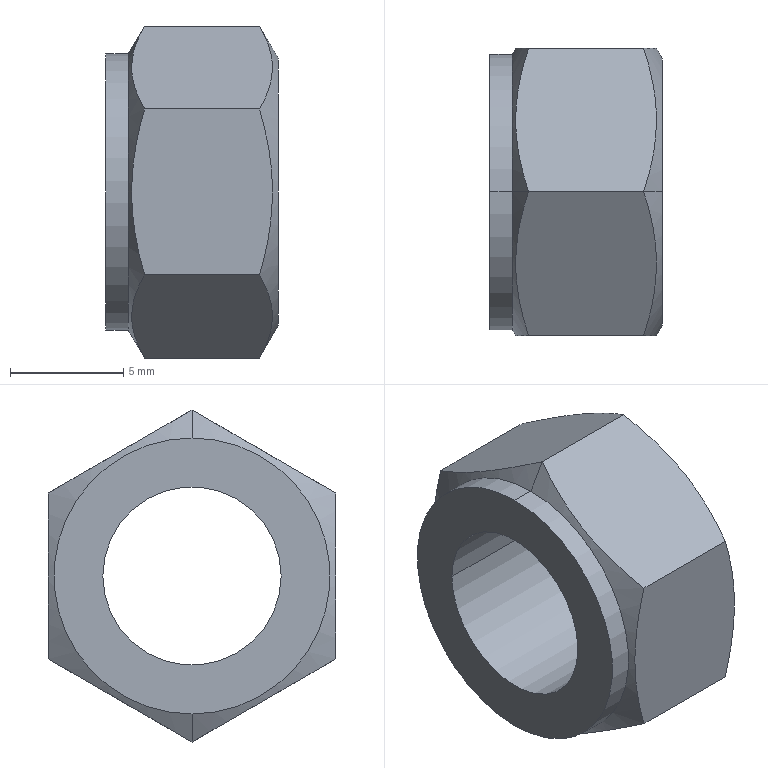Part | NX | features BREP 1 | 1 solid | 16 faces | box 7.62 x 12.7 x 14.665 mm | volume 657.652 mm3 | plane 8 | cylinder 4 | cone 4 | commonest cylinder face diameters 7.874 x2 12.192 x2
STEP:
#1=CARTESIAN_POINT('',(6.731,0.,5.903));
#2=VERTEX_POINT('',#1);
#3=CARTESIAN_POINT('',(6.731,0.,-5.903));
#4=VERTEX_POINT('',#3);
#5=CARTESIAN_POINT('',(6.731,0.,0.));
#6=DIRECTION('',(-1.,0.,0.));
#7=DIRECTION('',(0.,0.,1.));
#8=AXIS2_PLACEMENT_3D('',#5,#6,#7);
#9=CIRCLE('',#8,5.903);
#10=EDGE_CURVE('',#2,#4,#9,.T.);
#11=ORIENTED_EDGE('',*,*,#10,.F.);
#12=CARTESIAN_POINT('',(6.731,0.,0.));
#13=DIRECTION('',(-1.,0.,0.));
#14=DIRECTION('',(0.,0.,-1.));
#15=AXIS2_PLACEMENT_3D('',#12,#13,#14);
#16=CIRCLE('',#15,5.903);
#17=EDGE_CURVE('',#4,#2,#16,.T.);
#18=ORIENTED_EDGE('',*,*,#17,.F.);
#19=EDGE_LOOP('',(#11,#18));
#20=FACE_BOUND('',#19,.T.);
#21=CARTESIAN_POINT('',(6.731,-3.937,0.));
#22=VERTEX_POINT('',#21);
#23=CARTESIAN_POINT('',(6.731,3.937,0.));
#24=VERTEX_POINT('',#23);
#25=CARTESIAN_POINT('',(6.731,0.,0.));
#26=DIRECTION('',(1.,0.,0.));
#27=DIRECTION('',(0.,-1.,0.));
#28=AXIS2_PLACEMENT_3D('',#25,#26,#27);
#29=CIRCLE('',#28,3.937);
#30=EDGE_CURVE('',#22,#24,#29,.T.);
#31=ORIENTED_EDGE('',*,*,#30,.F.);
#32=CARTESIAN_POINT('',(6.731,0.,0.));
#33=DIRECTION('',(1.,0.,0.));
#34=DIRECTION('',(0.,1.,0.));
#35=AXIS2_PLACEMENT_3D('',#32,#33,#34);
#36=CIRCLE('',#35,3.937);
#37=EDGE_CURVE('',#24,#22,#36,.T.);
#38=ORIENTED_EDGE('',*,*,#37,.F.);
#39=EDGE_LOOP('',(#31,#38));
#40=FACE_BOUND('',#39,.T.);
#41=CARTESIAN_POINT('',(6.731,0.,0.));
#42=DIRECTION('',(1.,0.,0.));
#43=DIRECTION('',(0.,1.,0.));
#44=AXIS2_PLACEMENT_3D('',#41,#42,#43);
#45=PLANE('',#44);
#46=ADVANCED_FACE('',(#20,#40),#45,.T.);
#47=ORIENTED_EDGE('',*,*,#37,.T.);
#48=CARTESIAN_POINT('',(-0.889,-3.937,0.));
#49=VERTEX_POINT('',#48);
#50=CARTESIAN_POINT('',(-0.889,-3.937,0.));
#51=DIRECTION('',(1.,0.,0.));
#52=VECTOR('',#51,1000.);
#53=LINE('',#50,#52);
#54=EDGE_CURVE('',#22,#49,#53,.F.);
#55=ORIENTED_EDGE('',*,*,#54,.T.);
#56=CARTESIAN_POINT('',(-0.889,3.937,0.));
#57=VERTEX_POINT('',#56);
#58=CARTESIAN_POINT('',(-0.889,0.,0.));
#59=DIRECTION('',(1.,0.,0.));
#60=DIRECTION('',(0.,1.,0.));
#61=AXIS2_PLACEMENT_3D('',#58,#59,#60);
#62=CIRCLE('',#61,3.937);
#63=EDGE_CURVE('',#57,#49,#62,.T.);
#64=ORIENTED_EDGE('',*,*,#63,.F.);
#65=CARTESIAN_POINT('',(-0.889,3.937,0.));
#66=DIRECTION('',(1.,0.,0.));
#67=VECTOR('',#66,1000.);
#68=LINE('',#65,#67);
#69=EDGE_CURVE('',#24,#57,#68,.F.);
#70=ORIENTED_EDGE('',*,*,#69,.F.);
#71=EDGE_LOOP('',(#47,#55,#64,#70));
#72=FACE_BOUND('',#71,.T.);
#73=CARTESIAN_POINT('',(-1.651,0.,0.));
#74=DIRECTION('',(1.,0.,0.));
#75=DIRECTION('',(0.,1.,0.));
#76=AXIS2_PLACEMENT_3D('',#73,#74,#75);
#77=CYLINDRICAL_SURFACE('',#76,3.937);
#78=ADVANCED_FACE('',(#72),#77,.F.);
#79=CARTESIAN_POINT('',(-0.889,0.,0.));
#80=DIRECTION('',(1.,0.,0.));
#81=DIRECTION('',(0.,-1.,0.));
#82=AXIS2_PLACEMENT_3D('',#79,#80,#81);
#83=CIRCLE('',#82,3.937);
#84=EDGE_CURVE('',#49,#57,#83,.T.);
#85=ORIENTED_EDGE('',*,*,#84,.F.);
#86=ORIENTED_EDGE('',*,*,#54,.F.);
#87=ORIENTED_EDGE('',*,*,#30,.T.);
#88=ORIENTED_EDGE('',*,*,#69,.T.);
#89=EDGE_LOOP('',(#85,#86,#87,#88));
#90=FACE_BOUND('',#89,.T.);
#91=CARTESIAN_POINT('',(-1.651,0.,0.));
#92=DIRECTION('',(1.,0.,0.));
#93=DIRECTION('',(0.,1.,0.));
#94=AXIS2_PLACEMENT_3D('',#91,#92,#93);
#95=CYLINDRICAL_SURFACE('',#94,3.937);
#96=ADVANCED_FACE('',(#90),#95,.F.);
#97=CARTESIAN_POINT('',(-0.889,0.,6.096));
#98=VERTEX_POINT('',#97);
#99=CARTESIAN_POINT('',(-0.889,0.,-6.096));
#100=VERTEX_POINT('',#99);
#101=CARTESIAN_POINT('',(-0.889,0.,0.));
#102=DIRECTION('',(-1.,0.,0.));
#103=DIRECTION('',(0.,0.,1.));
#104=AXIS2_PLACEMENT_3D('',#101,#102,#103);
#105=CIRCLE('',#104,6.096);
#106=EDGE_CURVE('',#98,#100,#105,.T.);
#107=ORIENTED_EDGE('',*,*,#106,.T.);
#108=CARTESIAN_POINT('',(-0.889,0.,0.));
#109=DIRECTION('',(-1.,0.,0.));
#110=DIRECTION('',(0.,0.,-1.));
#111=AXIS2_PLACEMENT_3D('',#108,#109,#110);
#112=CIRCLE('',#111,6.096);
#113=EDGE_CURVE('',#100,#98,#112,.T.);
#114=ORIENTED_EDGE('',*,*,#113,.T.);
#115=EDGE_LOOP('',(#107,#114));
#116=FACE_BOUND('',#115,.T.);
#117=ORIENTED_EDGE('',*,*,#84,.T.);
#118=ORIENTED_EDGE('',*,*,#63,.T.);
#119=EDGE_LOOP('',(#117,#118));
#120=FACE_BOUND('',#119,.T.);
#121=CARTESIAN_POINT('',(-0.889,0.,0.));
#122=DIRECTION('',(-1.,0.,0.));
#123=DIRECTION('',(0.,0.,1.));
#124=AXIS2_PLACEMENT_3D('',#121,#122,#123);
#125=PLANE('',#124);
#126=ADVANCED_FACE('',(#116,#120),#125,.T.);
#127=CARTESIAN_POINT('',(0.1117,0.,6.096));
#128=VERTEX_POINT('',#127);
#129=CARTESIAN_POINT('',(0.1117,0.,6.096));
#130=DIRECTION('',(-1.,0.,0.));
#131=VECTOR('',#130,1000.);
#132=LINE('',#129,#131);
#133=EDGE_CURVE('',#98,#128,#132,.F.);
#134=ORIENTED_EDGE('',*,*,#133,.F.);
#135=ORIENTED_EDGE('',*,*,#113,.F.);
#136=CARTESIAN_POINT('',(0.1117,0.,-6.096));
#137=VERTEX_POINT('',#136);
#138=CARTESIAN_POINT('',(0.1117,0.,-6.096));
#139=DIRECTION('',(-1.,0.,0.));
#140=VECTOR('',#139,1000.);
#141=LINE('',#138,#140);
#142=EDGE_CURVE('',#100,#137,#141,.F.);
#143=ORIENTED_EDGE('',*,*,#142,.T.);
#144=CARTESIAN_POINT('',(0.1117,0.,0.));
#145=DIRECTION('',(-1.,0.,0.));
#146=DIRECTION('',(0.,0.,-1.));
#147=AXIS2_PLACEMENT_3D('',#144,#145,#146);
#148=CIRCLE('',#147,6.096);
#149=EDGE_CURVE('',#137,#128,#148,.T.);
#150=ORIENTED_EDGE('',*,*,#149,.T.);
#151=EDGE_LOOP('',(#134,#135,#143,#150));
#152=FACE_BOUND('',#151,.T.);
#153=CARTESIAN_POINT('',(0.508,0.,0.));
#154=DIRECTION('',(-1.,0.,0.));
#155=DIRECTION('',(0.,0.,-1.));
#156=AXIS2_PLACEMENT_3D('',#153,#154,#155);
#157=CYLINDRICAL_SURFACE('',#156,6.096);
#158=ADVANCED_FACE('',(#152),#157,.T.);
#159=CARTESIAN_POINT('',(0.8255,0.,-7.332));
#160=VERTEX_POINT('',#159);
#161=CARTESIAN_POINT('',(0.1117,0.,-6.096));
#162=DIRECTION('',(0.5,0.,-0.866));
#163=VECTOR('',#162,1000.);
#164=LINE('',#161,#163);
#165=EDGE_CURVE('',#137,#160,#164,.T.);
#166=ORIENTED_EDGE('',*,*,#165,.T.);
#167=CARTESIAN_POINT('',(0.8255,-6.35,-3.666));
#168=VERTEX_POINT('',#167);
#169=CARTESIAN_POINT('',(0.8255,-6.35,-3.666));
#170=CARTESIAN_POINT('',(0.07017,-4.084,-4.974));
#171=CARTESIAN_POINT('',(0.06957,-2.268,-6.023));
#172=CARTESIAN_POINT('',(0.8255,0.,-7.332));
#173=B_SPLINE_CURVE_WITH_KNOTS('',3,(#169,#170,#171,#172),.UNSPECIFIED.,.F.,.F.,(4,4),(0.,1.),.UNSPECIFIED.);
#174=EDGE_CURVE('',#160,#168,#173,.F.);
#175=ORIENTED_EDGE('',*,*,#174,.T.);
#176=CARTESIAN_POINT('',(0.8255,-6.35,3.666));
#177=VERTEX_POINT('',#176);
#178=CARTESIAN_POINT('',(0.8255,-6.35,3.666));
#179=CARTESIAN_POINT('',(0.07017,-6.35,1.05));
#180=CARTESIAN_POINT('',(0.06957,-6.35,-1.048));
#181=CARTESIAN_POINT('',(0.8255,-6.35,-3.666));
#182=B_SPLINE_CURVE_WITH_KNOTS('',3,(#178,#179,#180,#181),.UNSPECIFIED.,.F.,.F.,(4,4),(0.,1.),.UNSPECIFIED.);
#183=EDGE_CURVE('',#168,#177,#182,.F.);
#184=ORIENTED_EDGE('',*,*,#183,.T.);
#185=CARTESIAN_POINT('',(0.8255,0.,7.332));
#186=VERTEX_POINT('',#185);
#187=CARTESIAN_POINT('',(0.8255,0.,7.332));
#188=CARTESIAN_POINT('',(0.07017,-2.266,6.024));
#189=CARTESIAN_POINT('',(0.06957,-4.082,4.975));
#190=CARTESIAN_POINT('',(0.8255,-6.35,3.666));
#191=B_SPLINE_CURVE_WITH_KNOTS('',3,(#187,#188,#189,#190),.UNSPECIFIED.,.F.,.F.,(4,4),(0.,1.),.UNSPECIFIED.);
#192=EDGE_CURVE('',#177,#186,#191,.F.);
#193=ORIENTED_EDGE('',*,*,#192,.T.);
#194=CARTESIAN_POINT('',(0.1117,0.,6.096));
#195=DIRECTION('',(0.5,0.,0.866));
#196=VECTOR('',#195,1000.);
#197=LINE('',#194,#196);
#198=EDGE_CURVE('',#128,#186,#197,.T.);
#199=ORIENTED_EDGE('',*,*,#198,.F.);
#200=ORIENTED_EDGE('',*,*,#149,.F.);
#201=EDGE_LOOP('',(#166,#175,#184,#193,#199,#200));
#202=FACE_BOUND('',#201,.T.);
#203=CARTESIAN_POINT('',(0.4686,0.,0.));
#204=DIRECTION('',(1.,0.,0.));
#205=DIRECTION('',(0.,0.,1.));
#206=AXIS2_PLACEMENT_3D('',#203,#204,#205);
#207=CONICAL_SURFACE('',#206,6.714,1.047);
#208=ADVANCED_FACE('',(#202),#207,.T.);
#209=ORIENTED_EDGE('',*,*,#198,.T.);
#210=CARTESIAN_POINT('',(0.8255,6.35,3.666));
#211=VERTEX_POINT('',#210);
#212=CARTESIAN_POINT('',(0.8255,6.35,3.666));
#213=CARTESIAN_POINT('',(0.07017,4.084,4.974));
#214=CARTESIAN_POINT('',(0.06957,2.268,6.023));
#215=CARTESIAN_POINT('',(0.8255,0.,7.332));
#216=B_SPLINE_CURVE_WITH_KNOTS('',3,(#212,#213,#214,#215),.UNSPECIFIED.,.F.,.F.,(4,4),(0.,1.),.UNSPECIFIED.);
#217=EDGE_CURVE('',#186,#211,#216,.F.);
#218=ORIENTED_EDGE('',*,*,#217,.T.);
#219=CARTESIAN_POINT('',(0.8255,6.35,-3.666));
#220=VERTEX_POINT('',#219);
#221=CARTESIAN_POINT('',(0.8255,6.35,-3.666));
#222=CARTESIAN_POINT('',(0.07017,6.35,-1.05));
#223=CARTESIAN_POINT('',(0.06957,6.35,1.048));
#224=CARTESIAN_POINT('',(0.8255,6.35,3.666));
#225=B_SPLINE_CURVE_WITH_KNOTS('',3,(#221,#222,#223,#224),.UNSPECIFIED.,.F.,.F.,(4,4),(0.,1.),.UNSPECIFIED.);
#226=EDGE_CURVE('',#211,#220,#225,.F.);
#227=ORIENTED_EDGE('',*,*,#226,.T.);
#228=CARTESIAN_POINT('',(0.8255,0.,-7.332));
#229=CARTESIAN_POINT('',(0.07017,2.266,-6.024));
#230=CARTESIAN_POINT('',(0.06957,4.082,-4.975));
#231=CARTESIAN_POINT('',(0.8255,6.35,-3.666));
#232=B_SPLINE_CURVE_WITH_KNOTS('',3,(#228,#229,#230,#231),.UNSPECIFIED.,.F.,.F.,(4,4),(0.,1.),.UNSPECIFIED.);
#233=EDGE_CURVE('',#220,#160,#232,.F.);
#234=ORIENTED_EDGE('',*,*,#233,.T.);
#235=ORIENTED_EDGE('',*,*,#165,.F.);
#236=CARTESIAN_POINT('',(0.1117,0.,0.));
#237=DIRECTION('',(-1.,0.,0.));
#238=DIRECTION('',(0.,0.,1.));
#239=AXIS2_PLACEMENT_3D('',#236,#237,#238);
#240=CIRCLE('',#239,6.096);
#241=EDGE_CURVE('',#128,#137,#240,.T.);
#242=ORIENTED_EDGE('',*,*,#241,.F.);
#243=EDGE_LOOP('',(#209,#218,#227,#234,#235,#242));
#244=FACE_BOUND('',#243,.T.);
#245=CARTESIAN_POINT('',(0.4686,0.,0.));
#246=DIRECTION('',(1.,0.,0.));
#247=DIRECTION('',(0.,0.,1.));
#248=AXIS2_PLACEMENT_3D('',#245,#246,#247);
#249=CONICAL_SURFACE('',#248,6.714,1.047);
#250=ADVANCED_FACE('',(#244),#249,.T.);
#251=ORIENTED_EDGE('',*,*,#142,.F.);
#252=ORIENTED_EDGE('',*,*,#106,.F.);
#253=ORIENTED_EDGE('',*,*,#133,.T.);
#254=ORIENTED_EDGE('',*,*,#241,.T.);
#255=EDGE_LOOP('',(#251,#252,#253,#254));
#256=FACE_BOUND('',#255,.T.);
#257=CARTESIAN_POINT('',(0.508,0.,0.));
#258=DIRECTION('',(-1.,0.,0.));
#259=DIRECTION('',(0.,0.,-1.));
#260=AXIS2_PLACEMENT_3D('',#257,#258,#259);
#261=CYLINDRICAL_SURFACE('',#260,6.096);
#262=ADVANCED_FACE('',(#256),#261,.T.);
#263=CARTESIAN_POINT('',(5.905,0.,-7.332));
#264=VERTEX_POINT('',#263);
#265=CARTESIAN_POINT('',(0.8255,0.,-7.332));
#266=DIRECTION('',(1.,0.,0.));
#267=VECTOR('',#266,1000.);
#268=LINE('',#265,#267);
#269=EDGE_CURVE('',#160,#264,#268,.T.);
#270=ORIENTED_EDGE('',*,*,#269,.F.);
#271=ORIENTED_EDGE('',*,*,#233,.F.);
#272=CARTESIAN_POINT('',(5.905,6.35,-3.666));
#273=VERTEX_POINT('',#272);
#274=CARTESIAN_POINT('',(0.8255,6.35,-3.666));
#275=DIRECTION('',(1.,0.,0.));
#276=VECTOR('',#275,1000.);
#277=LINE('',#274,#276);
#278=EDGE_CURVE('',#220,#273,#277,.T.);
#279=ORIENTED_EDGE('',*,*,#278,.T.);
#280=CARTESIAN_POINT('',(5.905,6.35,-3.666));
#281=CARTESIAN_POINT('',(6.661,4.084,-4.974));
#282=CARTESIAN_POINT('',(6.662,2.268,-6.023));
#283=CARTESIAN_POINT('',(5.905,0.,-7.332));
#284=B_SPLINE_CURVE_WITH_KNOTS('',3,(#280,#281,#282,#283),.UNSPECIFIED.,.F.,.F.,(4,4),(0.,1.),.UNSPECIFIED.);
#285=EDGE_CURVE('',#273,#264,#284,.T.);
#286=ORIENTED_EDGE('',*,*,#285,.T.);
#287=EDGE_LOOP('',(#270,#271,#279,#286));
#288=FACE_BOUND('',#287,.T.);
#289=CARTESIAN_POINT('',(0.,0.,-7.332));
#290=DIRECTION('',(0.,0.5,-0.866));
#291=DIRECTION('',(-1.,0.,0.));
#292=AXIS2_PLACEMENT_3D('',#289,#290,#291);
#293=PLANE('',#292);
#294=ADVANCED_FACE('',(#288),#293,.T.);
#295=CARTESIAN_POINT('',(6.731,0.,-5.903));
#296=DIRECTION('',(-0.5,0.,-0.866));
#297=VECTOR('',#296,1000.);
#298=LINE('',#295,#297);
#299=EDGE_CURVE('',#4,#264,#298,.T.);
#300=ORIENTED_EDGE('',*,*,#299,.T.);
#301=ORIENTED_EDGE('',*,*,#285,.F.);
#302=CARTESIAN_POINT('',(5.905,6.35,3.666));
#303=VERTEX_POINT('',#302);
#304=CARTESIAN_POINT('',(5.905,6.35,3.666));
#305=CARTESIAN_POINT('',(6.661,6.35,1.05));
#306=CARTESIAN_POINT('',(6.662,6.35,-1.047));
#307=CARTESIAN_POINT('',(5.905,6.35,-3.666));
#308=B_SPLINE_CURVE_WITH_KNOTS('',3,(#304,#305,#306,#307),.UNSPECIFIED.,.F.,.F.,(4,4),(0.,1.),.UNSPECIFIED.);
#309=EDGE_CURVE('',#303,#273,#308,.T.);
#310=ORIENTED_EDGE('',*,*,#309,.F.);
#311=CARTESIAN_POINT('',(5.905,0.,7.332));
#312=VERTEX_POINT('',#311);
#313=CARTESIAN_POINT('',(5.905,0.,7.332));
#314=CARTESIAN_POINT('',(6.661,2.266,6.024));
#315=CARTESIAN_POINT('',(6.662,4.082,4.976));
#316=CARTESIAN_POINT('',(5.905,6.35,3.666));
#317=B_SPLINE_CURVE_WITH_KNOTS('',3,(#313,#314,#315,#316),.UNSPECIFIED.,.F.,.F.,(4,4),(0.,1.),.UNSPECIFIED.);
#318=EDGE_CURVE('',#312,#303,#317,.T.);
#319=ORIENTED_EDGE('',*,*,#318,.F.);
#320=CARTESIAN_POINT('',(6.731,0.,5.903));
#321=DIRECTION('',(-0.5,0.,0.866));
#322=VECTOR('',#321,1000.);
#323=LINE('',#320,#322);
#324=EDGE_CURVE('',#2,#312,#323,.T.);
#325=ORIENTED_EDGE('',*,*,#324,.F.);
#326=ORIENTED_EDGE('',*,*,#10,.T.);
#327=EDGE_LOOP('',(#300,#301,#310,#319,#325,#326));
#328=FACE_BOUND('',#327,.T.);
#329=CARTESIAN_POINT('',(6.318,0.,0.));
#330=DIRECTION('',(-1.,0.,0.));
#331=DIRECTION('',(0.,0.,-1.));
#332=AXIS2_PLACEMENT_3D('',#329,#330,#331);
#333=CONICAL_SURFACE('',#332,6.617,1.047);
#334=ADVANCED_FACE('',(#328),#333,.T.);
#335=ORIENTED_EDGE('',*,*,#324,.T.);
#336=CARTESIAN_POINT('',(5.905,-6.35,3.666));
#337=VERTEX_POINT('',#336);
#338=CARTESIAN_POINT('',(5.905,-6.35,3.666));
#339=CARTESIAN_POINT('',(6.661,-4.084,4.974));
#340=CARTESIAN_POINT('',(6.662,-2.268,6.023));
#341=CARTESIAN_POINT('',(5.905,0.,7.332));
#342=B_SPLINE_CURVE_WITH_KNOTS('',3,(#338,#339,#340,#341),.UNSPECIFIED.,.F.,.F.,(4,4),(0.,1.),.UNSPECIFIED.);
#343=EDGE_CURVE('',#337,#312,#342,.T.);
#344=ORIENTED_EDGE('',*,*,#343,.F.);
#345=CARTESIAN_POINT('',(5.905,-6.35,-3.666));
#346=VERTEX_POINT('',#345);
#347=CARTESIAN_POINT('',(5.905,-6.35,-3.666));
#348=CARTESIAN_POINT('',(6.661,-6.35,-1.05));
#349=CARTESIAN_POINT('',(6.662,-6.35,1.047));
#350=CARTESIAN_POINT('',(5.905,-6.35,3.666));
#351=B_SPLINE_CURVE_WITH_KNOTS('',3,(#347,#348,#349,#350),.UNSPECIFIED.,.F.,.F.,(4,4),(0.,1.),.UNSPECIFIED.);
#352=EDGE_CURVE('',#346,#337,#351,.T.);
#353=ORIENTED_EDGE('',*,*,#352,.F.);
#354=CARTESIAN_POINT('',(5.905,0.,-7.332));
#355=CARTESIAN_POINT('',(6.661,-2.266,-6.024));
#356=CARTESIAN_POINT('',(6.662,-4.082,-4.976));
#357=CARTESIAN_POINT('',(5.905,-6.35,-3.666));
#358=B_SPLINE_CURVE_WITH_KNOTS('',3,(#354,#355,#356,#357),.UNSPECIFIED.,.F.,.F.,(4,4),(0.,1.),.UNSPECIFIED.);
#359=EDGE_CURVE('',#264,#346,#358,.T.);
#360=ORIENTED_EDGE('',*,*,#359,.F.);
#361=ORIENTED_EDGE('',*,*,#299,.F.);
#362=ORIENTED_EDGE('',*,*,#17,.T.);
#363=EDGE_LOOP('',(#335,#344,#353,#360,#361,#362));
#364=FACE_BOUND('',#363,.T.);
#365=CARTESIAN_POINT('',(6.318,0.,0.));
#366=DIRECTION('',(-1.,0.,0.));
#367=DIRECTION('',(0.,0.,-1.));
#368=AXIS2_PLACEMENT_3D('',#365,#366,#367);
#369=CONICAL_SURFACE('',#368,6.617,1.047);
#370=ADVANCED_FACE('',(#364),#369,.T.);
#371=CARTESIAN_POINT('',(0.8255,-6.35,-3.666));
#372=DIRECTION('',(1.,0.,0.));
#373=VECTOR('',#372,1000.);
#374=LINE('',#371,#373);
#375=EDGE_CURVE('',#168,#346,#374,.T.);
#376=ORIENTED_EDGE('',*,*,#375,.F.);
#377=ORIENTED_EDGE('',*,*,#174,.F.);
#378=ORIENTED_EDGE('',*,*,#269,.T.);
#379=ORIENTED_EDGE('',*,*,#359,.T.);
#380=EDGE_LOOP('',(#376,#377,#378,#379));
#381=FACE_BOUND('',#380,.T.);
#382=CARTESIAN_POINT('',(0.,-6.35,-3.666));
#383=DIRECTION('',(0.,-0.5,-0.866));
#384=DIRECTION('',(0.,-0.866,0.5));
#385=AXIS2_PLACEMENT_3D('',#382,#383,#384);
#386=PLANE('',#385);
#387=ADVANCED_FACE('',(#381),#386,.T.);
#388=CARTESIAN_POINT('',(0.8255,-6.35,3.666));
#389=DIRECTION('',(1.,0.,0.));
#390=VECTOR('',#389,1000.);
#391=LINE('',#388,#390);
#392=EDGE_CURVE('',#177,#337,#391,.T.);
#393=ORIENTED_EDGE('',*,*,#392,.F.);
#394=ORIENTED_EDGE('',*,*,#183,.F.);
#395=ORIENTED_EDGE('',*,*,#375,.T.);
#396=ORIENTED_EDGE('',*,*,#352,.T.);
#397=EDGE_LOOP('',(#393,#394,#395,#396));
#398=FACE_BOUND('',#397,.T.);
#399=CARTESIAN_POINT('',(0.,-6.35,3.666));
#400=DIRECTION('',(0.,-1.,0.));
#401=DIRECTION('',(0.,0.,-1.));
#402=AXIS2_PLACEMENT_3D('',#399,#400,#401);
#403=PLANE('',#402);
#404=ADVANCED_FACE('',(#398),#403,.T.);
#405=CARTESIAN_POINT('',(0.8255,0.,7.332));
#406=DIRECTION('',(1.,0.,0.));
#407=VECTOR('',#406,1000.);
#408=LINE('',#405,#407);
#409=EDGE_CURVE('',#186,#312,#408,.T.);
#410=ORIENTED_EDGE('',*,*,#409,.F.);
#411=ORIENTED_EDGE('',*,*,#192,.F.);
#412=ORIENTED_EDGE('',*,*,#392,.T.);
#413=ORIENTED_EDGE('',*,*,#343,.T.);
#414=EDGE_LOOP('',(#410,#411,#412,#413));
#415=FACE_BOUND('',#414,.T.);
#416=CARTESIAN_POINT('',(0.,0.,7.332));
#417=DIRECTION('',(0.,-0.5,0.866));
#418=DIRECTION('',(-1.,0.,0.));
#419=AXIS2_PLACEMENT_3D('',#416,#417,#418);
#420=PLANE('',#419);
#421=ADVANCED_FACE('',(#415),#420,.T.);
#422=CARTESIAN_POINT('',(0.8255,6.35,3.666));
#423=DIRECTION('',(1.,0.,0.));
#424=VECTOR('',#423,1000.);
#425=LINE('',#422,#424);
#426=EDGE_CURVE('',#211,#303,#425,.T.);
#427=ORIENTED_EDGE('',*,*,#426,.F.);
#428=ORIENTED_EDGE('',*,*,#217,.F.);
#429=ORIENTED_EDGE('',*,*,#409,.T.);
#430=ORIENTED_EDGE('',*,*,#318,.T.);
#431=EDGE_LOOP('',(#427,#428,#429,#430));
#432=FACE_BOUND('',#431,.T.);
#433=CARTESIAN_POINT('',(0.,6.35,3.666));
#434=DIRECTION('',(0.,0.5,0.866));
#435=DIRECTION('',(1.,0.,0.));
#436=AXIS2_PLACEMENT_3D('',#433,#434,#435);
#437=PLANE('',#436);
#438=ADVANCED_FACE('',(#432),#437,.T.);
#439=ORIENTED_EDGE('',*,*,#278,.F.);
#440=ORIENTED_EDGE('',*,*,#226,.F.);
#441=ORIENTED_EDGE('',*,*,#426,.T.);
#442=ORIENTED_EDGE('',*,*,#309,.T.);
#443=EDGE_LOOP('',(#439,#440,#441,#442));
#444=FACE_BOUND('',#443,.T.);
#445=CARTESIAN_POINT('',(0.,6.35,-3.666));
#446=DIRECTION('',(0.,1.,0.));
#447=DIRECTION('',(1.,0.,0.));
#448=AXIS2_PLACEMENT_3D('',#445,#446,#447);
#449=PLANE('',#448);
#450=ADVANCED_FACE('',(#444),#449,.T.);
#451=CLOSED_SHELL('',(#46,#78,#96,#126,#158,#208,#250,#262,#294,#334,#370,#387,#404,#421,#438,#450));
#452=MANIFOLD_SOLID_BREP('',#451);
#453=(LENGTH_UNIT()NAMED_UNIT(*)SI_UNIT(.MILLI.,.METRE.));
#454=UNCERTAINTY_MEASURE_WITH_UNIT(LENGTH_MEASURE(0.0508),#453,'','');
#455=(NAMED_UNIT(*)PLANE_ANGLE_UNIT()SI_UNIT($,.RADIAN.));
#456=(NAMED_UNIT(*)SI_UNIT($,.STERADIAN.)SOLID_ANGLE_UNIT());
#457=(GEOMETRIC_REPRESENTATION_CONTEXT(3)GLOBAL_UNCERTAINTY_ASSIGNED_CONTEXT((#454))GLOBAL_UNIT_ASSIGNED_CONTEXT((#453,#455,#456))REPRESENTATION_CONTEXT('',''));
#458=ADVANCED_BREP_SHAPE_REPRESENTATION('',(#452),#457);